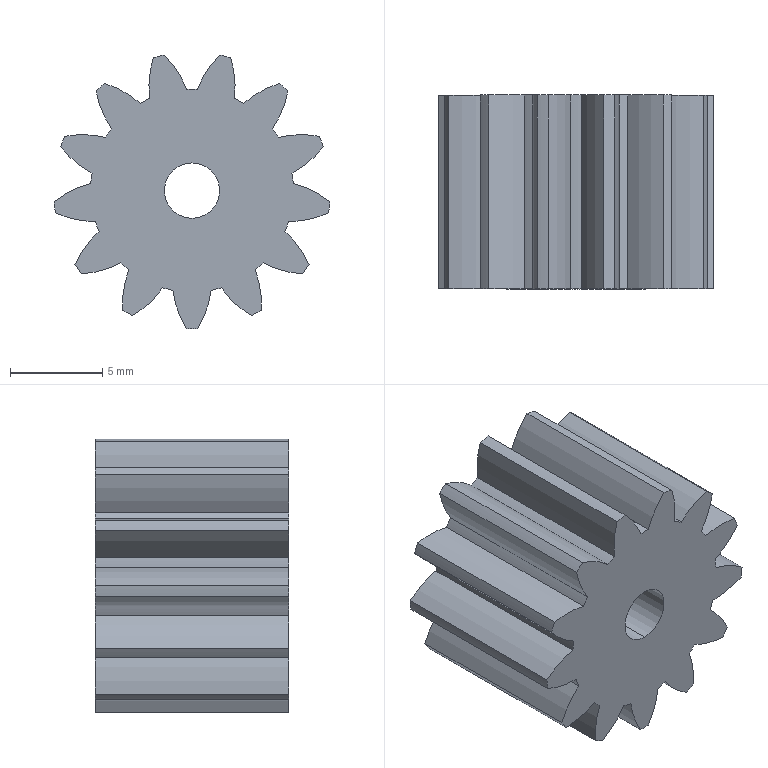Part | SolidWorks | features Extrusion 1, ICE 1 | 1 solid | 57 faces | box 14.953 x 10.5 x 14.85 mm | volume 1337 mm3 | cylinder 55 | plane 2 | commonest cylinder face diameters 10.8 x26 15 x14 11 x13 3 x2